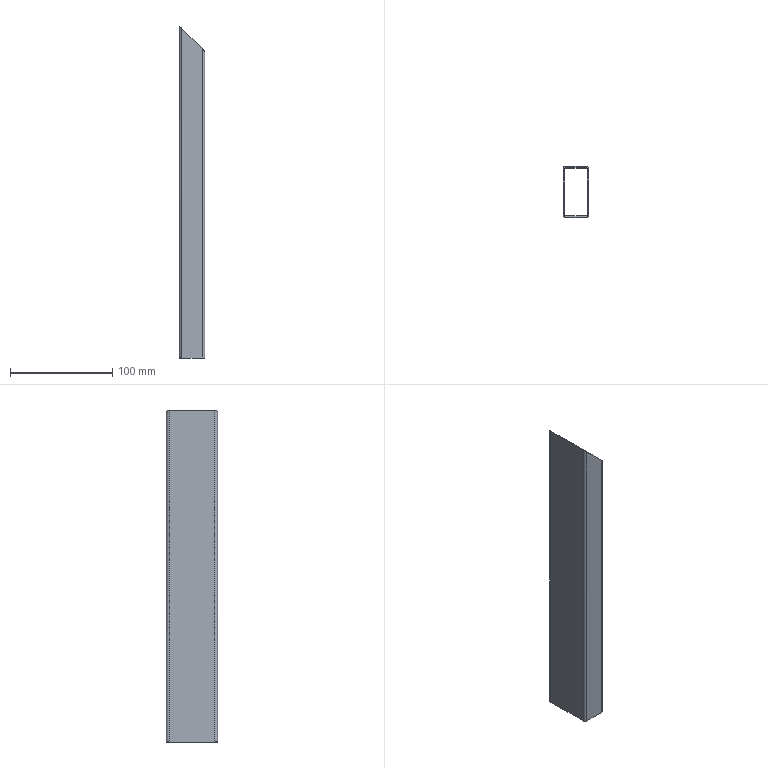Part | STEP file | 7100515 | 1 solid | 18 faces | box 25 x 50 x 325 mm | volume 66092 mm3 | plane 10 | cylinder 8 | commonest cylinder face diameters 2 x4 5 x4